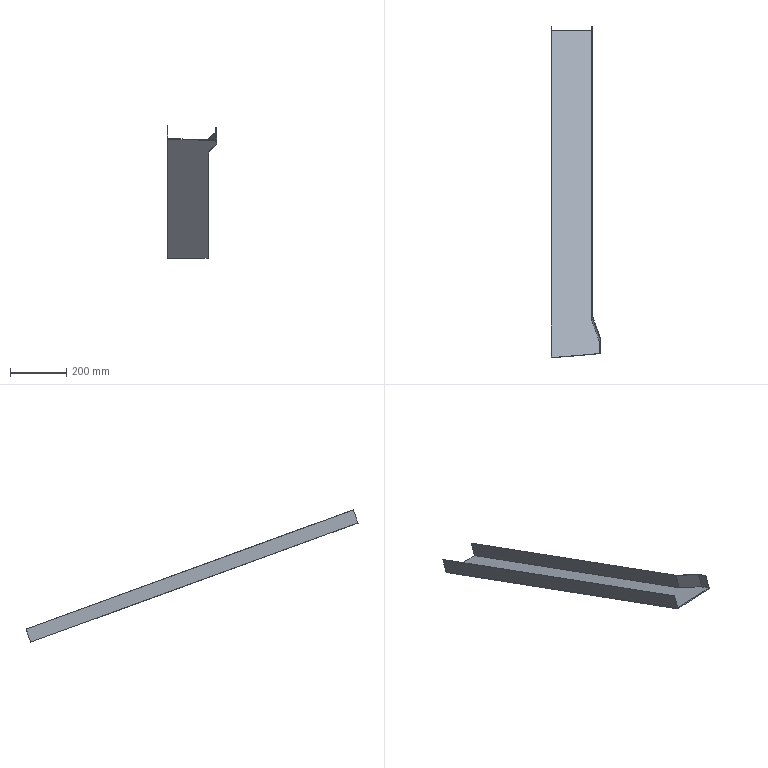Part | NX | features solid 2 | 1 solid | 20 faces | box 175.737 x 1183 x 471.211 mm | volume 600196 mm3 | plane 13 | spline 7
STEP:
#1=CARTESIAN_POINT('',(-1118.,-193.74,-135.956));
#2=VERTEX_POINT('',#1);
#3=CARTESIAN_POINT('',(-1118.,971.638,-560.119));
#4=VERTEX_POINT('',#3);
#5=CARTESIAN_POINT('',(-1118.,-136.156,-156.914));
#6=DIRECTION('',(0.,0.9397,-0.342));
#7=VECTOR('',#6,1000.);
#8=LINE('',#5,#7);
#9=EDGE_CURVE('',#2,#4,#8,.T.);
#10=ORIENTED_EDGE('',*,*,#9,.F.);
#11=CARTESIAN_POINT('',(-945.824,-178.677,-141.438));
#12=VERTEX_POINT('',#11);
#13=CARTESIAN_POINT('',(-1218.424,-202.526,-132.758));
#14=DIRECTION('',(0.9957,0.08711,-0.03171));
#15=VECTOR('',#14,1000.);
#16=LINE('',#13,#15);
#17=EDGE_CURVE('',#2,#12,#16,.T.);
#18=ORIENTED_EDGE('',*,*,#17,.T.);
#19=CARTESIAN_POINT('',(-947.819,-178.548,-141.485));
#20=VERTEX_POINT('',#19);
#21=CARTESIAN_POINT('',(-1226.783,-160.524,-148.045));
#22=DIRECTION('',(0.9976,-0.06446,0.02346));
#23=VECTOR('',#22,1000.);
#24=LINE('',#21,#23);
#25=EDGE_CURVE('',#20,#12,#24,.T.);
#26=ORIENTED_EDGE('',*,*,#25,.F.);
#27=CARTESIAN_POINT('',(-946.331,-142.065,-154.764));
#28=VERTEX_POINT('',#27);
#29=CARTESIAN_POINT('',(-947.819,-178.548,-141.485));
#30=CARTESIAN_POINT('',(-947.597,-175.511,-142.591));
#31=CARTESIAN_POINT('',(-946.951,-169.452,-144.796));
#32=CARTESIAN_POINT('',(-946.188,-157.291,-149.222));
#33=CARTESIAN_POINT('',(-946.239,-148.154,-152.548));
#34=CARTESIAN_POINT('',(-946.331,-142.065,-154.764));
#35=B_SPLINE_CURVE_WITH_KNOTS('',3,(#29,#30,#31,#32,#33,#34),.UNSPECIFIED.,.F.,.F.,(4,1,1,4),(0.,0.009718,0.01944,0.03887),.UNSPECIFIED.);
#36=EDGE_CURVE('',#20,#28,#35,.T.);
#37=ORIENTED_EDGE('',*,*,#36,.T.);
#38=CARTESIAN_POINT('',(-977.,-57.802,-185.433));
#39=VERTEX_POINT('',#38);
#40=CARTESIAN_POINT('',(-977.44,-56.592,-185.873));
#41=DIRECTION('',(-0.3236,0.8891,-0.3236));
#42=VECTOR('',#41,1000.);
#43=LINE('',#40,#42);
#44=EDGE_CURVE('',#28,#39,#43,.T.);
#45=ORIENTED_EDGE('',*,*,#44,.T.);
#46=CARTESIAN_POINT('',(-977.,971.638,-560.119));
#47=VERTEX_POINT('',#46);
#48=CARTESIAN_POINT('',(-977.,-136.156,-156.914));
#49=DIRECTION('',(0.,0.9397,-0.342));
#50=VECTOR('',#49,1000.);
#51=LINE('',#48,#50);
#52=EDGE_CURVE('',#39,#47,#51,.T.);
#53=ORIENTED_EDGE('',*,*,#52,.T.);
#54=CARTESIAN_POINT('',(-1100.,971.638,-560.119));
#55=DIRECTION('',(1.,0.,0.));
#56=VECTOR('',#55,1000.);
#57=LINE('',#54,#56);
#58=EDGE_CURVE('',#4,#47,#57,.T.);
#59=ORIENTED_EDGE('',*,*,#58,.F.);
#60=EDGE_LOOP('',(#10,#18,#26,#37,#45,#53,#59));
#61=FACE_BOUND('',#60,.T.);
#62=CARTESIAN_POINT('',(-1225.,-136.156,-156.914));
#63=DIRECTION('',(0.,-0.342,-0.9397));
#64=DIRECTION('',(0.,0.9397,-0.342));
#65=AXIS2_PLACEMENT_3D('',#62,#63,#64);
#66=PLANE('',#65);
#67=ADVANCED_FACE('',(#61),#66,.F.);
#68=CARTESIAN_POINT('',(-1118.,-194.424,-137.835));
#69=VERTEX_POINT('',#68);
#70=CARTESIAN_POINT('',(-1118.,-194.424,-137.835));
#71=DIRECTION('',(0.,0.342,0.9397));
#72=VECTOR('',#71,1000.);
#73=LINE('',#70,#72);
#74=EDGE_CURVE('',#69,#2,#73,.T.);
#75=ORIENTED_EDGE('',*,*,#74,.F.);
#76=CARTESIAN_POINT('',(-945.824,-179.361,-143.318));
#77=VERTEX_POINT('',#76);
#78=CARTESIAN_POINT('',(-1218.424,-203.21,-134.637));
#79=DIRECTION('',(0.9957,0.08711,-0.03171));
#80=VECTOR('',#79,1000.);
#81=LINE('',#78,#80);
#82=EDGE_CURVE('',#69,#77,#81,.T.);
#83=ORIENTED_EDGE('',*,*,#82,.T.);
#84=CARTESIAN_POINT('',(-945.824,-179.019,-142.378));
#85=DIRECTION('',(0.,0.342,0.9397));
#86=VECTOR('',#85,1000.);
#87=LINE('',#84,#86);
#88=EDGE_CURVE('',#77,#12,#87,.T.);
#89=ORIENTED_EDGE('',*,*,#88,.T.);
#90=ORIENTED_EDGE('',*,*,#17,.F.);
#91=EDGE_LOOP('',(#75,#83,#89,#90));
#92=FACE_BOUND('',#91,.T.);
#93=CARTESIAN_POINT('',(-1218.424,-203.21,-134.637));
#94=DIRECTION('',(-0.0927,0.9356,-0.3405));
#95=DIRECTION('',(0.,0.342,0.9397));
#96=AXIS2_PLACEMENT_3D('',#93,#94,#95);
#97=PLANE('',#96);
#98=ADVANCED_FACE('',(#92),#97,.F.);
#99=CARTESIAN_POINT('',(-944.358,-157.689,-149.077));
#100=VERTEX_POINT('',#99);
#101=CARTESIAN_POINT('',(-944.358,-158.364,-150.96));
#102=VERTEX_POINT('',#101);
#103=CARTESIAN_POINT('',(-944.358,-141.272,-103.972));
#104=DIRECTION('',(0.,-0.342,-0.9397));
#105=VECTOR('',#104,1000.);
#106=LINE('',#103,#105);
#107=EDGE_CURVE('',#100,#102,#106,.T.);
#108=ORIENTED_EDGE('',*,*,#107,.F.);
#109=CARTESIAN_POINT('',(-945.,-169.316,-144.845));
#110=VERTEX_POINT('',#109);
#111=CARTESIAN_POINT('',(-945.,-169.316,-144.845));
#112=CARTESIAN_POINT('',(-944.911,-168.24,-145.237));
#113=CARTESIAN_POINT('',(-944.751,-166.152,-145.997));
#114=CARTESIAN_POINT('',(-944.614,-164.006,-146.778));
#115=CARTESIAN_POINT('',(-944.536,-162.589,-147.294));
#116=CARTESIAN_POINT('',(-944.496,-161.793,-147.584));
#117=CARTESIAN_POINT('',(-944.431,-160.279,-148.135));
#118=CARTESIAN_POINT('',(-944.385,-158.779,-148.68));
#119=CARTESIAN_POINT('',(-944.358,-157.689,-149.077));
#120=B_SPLINE_CURVE_WITH_KNOTS('',3,(#111,#112,#113,#114,#115,#116,#117,#118,#119),.UNSPECIFIED.,.F.,.F.,(4,1,1,1,1,1,4),(0.,0.1082,0.2163,0.2434,0.2704,0.3245,0.4327),.UNSPECIFIED.);
#121=EDGE_CURVE('',#110,#100,#120,.T.);
#122=ORIENTED_EDGE('',*,*,#121,.F.);
#123=CARTESIAN_POINT('',(-945.,-170.,-146.725));
#124=VERTEX_POINT('',#123);
#125=CARTESIAN_POINT('',(-945.,-170.,-146.725));
#126=CARTESIAN_POINT('',(-945.,-169.772,-146.098));
#127=CARTESIAN_POINT('',(-945.,-169.544,-145.472));
#128=CARTESIAN_POINT('',(-945.,-169.316,-144.845));
#129=B_SPLINE_CURVE_WITH_KNOTS('',3,(#125,#126,#127,#128),.UNSPECIFIED.,.F.,.F.,(4,4),(0.,1.),.UNSPECIFIED.);
#130=EDGE_CURVE('',#124,#110,#129,.T.);
#131=ORIENTED_EDGE('',*,*,#130,.F.);
#132=CARTESIAN_POINT('',(-945.,-170.,-146.725));
#133=CARTESIAN_POINT('',(-944.911,-168.923,-147.117));
#134=CARTESIAN_POINT('',(-944.751,-166.834,-147.877));
#135=CARTESIAN_POINT('',(-944.613,-164.687,-148.659));
#136=CARTESIAN_POINT('',(-944.536,-163.269,-149.175));
#137=CARTESIAN_POINT('',(-944.496,-162.473,-149.464));
#138=CARTESIAN_POINT('',(-944.431,-160.956,-150.016));
#139=CARTESIAN_POINT('',(-944.385,-159.455,-150.563));
#140=CARTESIAN_POINT('',(-944.358,-158.364,-150.96));
#141=B_SPLINE_CURVE_WITH_KNOTS('',3,(#132,#133,#134,#135,#136,#137,#138,#139,#140),.UNSPECIFIED.,.F.,.F.,(4,1,1,1,1,1,4),(0.,0.1082,0.2165,0.2435,0.2706,0.3247,0.433),.UNSPECIFIED.);
#142=EDGE_CURVE('',#102,#124,#141,.F.);
#143=ORIENTED_EDGE('',*,*,#142,.F.);
#144=EDGE_LOOP('',(#108,#122,#131,#143));
#145=FACE_BOUND('',#144,.T.);
#146=CARTESIAN_POINT('',(-945.,-170.,-146.725));
#147=CARTESIAN_POINT('',(-945.,-169.316,-144.845));
#148=CARTESIAN_POINT('',(-944.91,-168.917,-147.119));
#149=CARTESIAN_POINT('',(-944.91,-168.233,-145.24));
#150=CARTESIAN_POINT('',(-944.749,-166.815,-147.884));
#151=CARTESIAN_POINT('',(-944.749,-166.131,-146.005));
#152=CARTESIAN_POINT('',(-944.612,-164.658,-148.669));
#153=CARTESIAN_POINT('',(-944.612,-163.974,-146.79));
#154=CARTESIAN_POINT('',(-944.534,-163.231,-149.188));
#155=CARTESIAN_POINT('',(-944.534,-162.547,-147.309));
#156=CARTESIAN_POINT('',(-944.494,-162.438,-149.477));
#157=CARTESIAN_POINT('',(-944.494,-161.754,-147.598));
#158=CARTESIAN_POINT('',(-944.429,-160.9,-150.037));
#159=CARTESIAN_POINT('',(-944.429,-160.216,-148.157));
#160=CARTESIAN_POINT('',(-944.383,-159.388,-150.587));
#161=CARTESIAN_POINT('',(-944.383,-158.704,-148.708));
#162=CARTESIAN_POINT('',(-944.356,-158.286,-150.988));
#163=CARTESIAN_POINT('',(-944.356,-157.602,-149.109));
#164=B_SPLINE_SURFACE_WITH_KNOTS('',3,1,((#146,#147),(#148,#149),(#150,#151),(#152,#153),(#154,#155),(#156,#157),(#158,#159),(#160,#161),(#162,#163)),.SURF_OF_LINEAR_EXTRUSION.,.F.,.F.,.F.,(4,1,1,1,1,1,4),(2,2),(0.,0.1089,0.2178,0.245,0.2722,0.3267,0.4356),(0.,1.),.UNSPECIFIED.);
#165=ADVANCED_FACE('',(#145),#164,.T.);
#166=CARTESIAN_POINT('',(-975.,-58.173,-187.426));
#167=VERTEX_POINT('',#166);
#168=CARTESIAN_POINT('',(-975.,-41.072,-140.442));
#169=VERTEX_POINT('',#168);
#170=CARTESIAN_POINT('',(-975.,-58.173,-187.426));
#171=DIRECTION('',(0.,0.342,0.9397));
#172=VECTOR('',#171,1000.);
#173=LINE('',#170,#172);
#174=EDGE_CURVE('',#167,#169,#173,.T.);
#175=ORIENTED_EDGE('',*,*,#174,.T.);
#176=CARTESIAN_POINT('',(-944.335,-125.322,-109.777));
#177=VERTEX_POINT('',#176);
#178=CARTESIAN_POINT('',(-944.335,-125.322,-109.777));
#179=CARTESIAN_POINT('',(-954.557,-97.239,-119.999));
#180=CARTESIAN_POINT('',(-964.778,-69.155,-130.22));
#181=CARTESIAN_POINT('',(-975.,-41.072,-140.442));
#182=B_SPLINE_CURVE_WITH_KNOTS('',3,(#178,#179,#180,#181),.UNSPECIFIED.,.F.,.F.,(4,4),(0.03202,0.1091),.PIECEWISE_BEZIER_KNOTS.);
#183=EDGE_CURVE('',#177,#169,#182,.T.);
#184=ORIENTED_EDGE('',*,*,#183,.F.);
#185=CARTESIAN_POINT('',(-944.335,-141.739,-154.883));
#186=VERTEX_POINT('',#185);
#187=CARTESIAN_POINT('',(-944.335,-125.322,-109.777));
#188=DIRECTION('',(0.,-0.342,-0.9397));
#189=VECTOR('',#188,1000.);
#190=LINE('',#187,#189);
#191=EDGE_CURVE('',#177,#186,#190,.T.);
#192=ORIENTED_EDGE('',*,*,#191,.T.);
#193=CARTESIAN_POINT('',(-944.335,-142.423,-156.762));
#194=VERTEX_POINT('',#193);
#195=CARTESIAN_POINT('',(-944.335,-142.423,-156.762));
#196=CARTESIAN_POINT('',(-944.335,-142.195,-156.135));
#197=CARTESIAN_POINT('',(-944.335,-141.967,-155.509));
#198=CARTESIAN_POINT('',(-944.335,-141.739,-154.883));
#199=B_SPLINE_CURVE_WITH_KNOTS('',3,(#195,#196,#197,#198),.UNSPECIFIED.,.F.,.F.,(4,4),(0.,1.),.UNSPECIFIED.);
#200=EDGE_CURVE('',#186,#194,#199,.F.);
#201=ORIENTED_EDGE('',*,*,#200,.T.);
#202=CARTESIAN_POINT('',(-975.548,-56.668,-187.974));
#203=DIRECTION('',(-0.3236,0.8891,-0.3236));
#204=VECTOR('',#203,1000.);
#205=LINE('',#202,#204);
#206=EDGE_CURVE('',#194,#167,#205,.T.);
#207=ORIENTED_EDGE('',*,*,#206,.T.);
#208=EDGE_LOOP('',(#175,#184,#192,#201,#207));
#209=FACE_BOUND('',#208,.T.);
#210=CARTESIAN_POINT('',(-975.548,-56.668,-187.974));
#211=DIRECTION('',(0.9462,0.3041,-0.1107));
#212=DIRECTION('',(-0.306,0.952,0.));
#213=AXIS2_PLACEMENT_3D('',#210,#211,#212);
#214=PLANE('',#213);
#215=ADVANCED_FACE('',(#209),#214,.T.);
#216=CARTESIAN_POINT('',(-975.,970.954,-561.998));
#217=VERTEX_POINT('',#216);
#218=CARTESIAN_POINT('',(-975.,988.055,-515.013));
#219=VERTEX_POINT('',#218);
#220=CARTESIAN_POINT('',(-975.,970.954,-561.998));
#221=DIRECTION('',(0.,0.342,0.9397));
#222=VECTOR('',#221,1000.);
#223=LINE('',#220,#222);
#224=EDGE_CURVE('',#217,#219,#223,.T.);
#225=ORIENTED_EDGE('',*,*,#224,.T.);
#226=CARTESIAN_POINT('',(-975.,-41.072,-140.442));
#227=CARTESIAN_POINT('',(-975.,301.97,-265.299));
#228=CARTESIAN_POINT('',(-975.,645.013,-390.156));
#229=CARTESIAN_POINT('',(-975.,988.055,-515.013));
#230=B_SPLINE_CURVE_WITH_KNOTS('',3,(#226,#227,#228,#229),.UNSPECIFIED.,.F.,.F.,(4,4),(0.1091,1.),.PIECEWISE_BEZIER_KNOTS.);
#231=EDGE_CURVE('',#169,#219,#230,.T.);
#232=ORIENTED_EDGE('',*,*,#231,.F.);
#233=ORIENTED_EDGE('',*,*,#174,.F.);
#234=CARTESIAN_POINT('',(-975.,-136.84,-158.794));
#235=DIRECTION('',(0.,0.9397,-0.342));
#236=VECTOR('',#235,1000.);
#237=LINE('',#234,#236);
#238=EDGE_CURVE('',#167,#217,#237,.T.);
#239=ORIENTED_EDGE('',*,*,#238,.T.);
#240=EDGE_LOOP('',(#225,#232,#233,#239));
#241=FACE_BOUND('',#240,.T.);
#242=CARTESIAN_POINT('',(-975.,-136.84,-158.794));
#243=DIRECTION('',(1.,0.,0.));
#244=DIRECTION('',(0.,0.,-1.));
#245=AXIS2_PLACEMENT_3D('',#242,#243,#244);
#246=PLANE('',#245);
#247=ADVANCED_FACE('',(#241),#246,.T.);
#248=CARTESIAN_POINT('',(-1120.,970.954,-561.998));
#249=VERTEX_POINT('',#248);
#250=CARTESIAN_POINT('',(-1120.,988.055,-515.013));
#251=VERTEX_POINT('',#250);
#252=CARTESIAN_POINT('',(-1120.,970.954,-561.998));
#253=DIRECTION('',(0.,0.342,0.9397));
#254=VECTOR('',#253,1000.);
#255=LINE('',#252,#254);
#256=EDGE_CURVE('',#249,#251,#255,.T.);
#257=ORIENTED_EDGE('',*,*,#256,.T.);
#258=CARTESIAN_POINT('',(-1118.,988.055,-515.013));
#259=VERTEX_POINT('',#258);
#260=CARTESIAN_POINT('',(-1120.,988.055,-515.013));
#261=DIRECTION('',(1.,0.,0.));
#262=VECTOR('',#261,1000.);
#263=LINE('',#260,#262);
#264=EDGE_CURVE('',#251,#259,#263,.T.);
#265=ORIENTED_EDGE('',*,*,#264,.T.);
#266=CARTESIAN_POINT('',(-1118.,988.055,-515.013));
#267=DIRECTION('',(0.,-0.342,-0.9397));
#268=VECTOR('',#267,1000.);
#269=LINE('',#266,#268);
#270=EDGE_CURVE('',#259,#4,#269,.T.);
#271=ORIENTED_EDGE('',*,*,#270,.T.);
#272=ORIENTED_EDGE('',*,*,#58,.T.);
#273=CARTESIAN_POINT('',(-977.,988.055,-515.013));
#274=VERTEX_POINT('',#273);
#275=CARTESIAN_POINT('',(-977.,988.055,-515.013));
#276=DIRECTION('',(0.,-0.342,-0.9397));
#277=VECTOR('',#276,1000.);
#278=LINE('',#275,#277);
#279=EDGE_CURVE('',#274,#47,#278,.T.);
#280=ORIENTED_EDGE('',*,*,#279,.F.);
#281=CARTESIAN_POINT('',(-975.,988.055,-515.013));
#282=DIRECTION('',(1.,0.,0.));
#283=VECTOR('',#282,1000.);
#284=LINE('',#281,#283);
#285=EDGE_CURVE('',#219,#274,#284,.F.);
#286=ORIENTED_EDGE('',*,*,#285,.F.);
#287=ORIENTED_EDGE('',*,*,#224,.F.);
#288=CARTESIAN_POINT('',(-1100.,970.954,-561.998));
#289=DIRECTION('',(1.,0.,0.));
#290=VECTOR('',#289,1000.);
#291=LINE('',#288,#290);
#292=EDGE_CURVE('',#249,#217,#291,.T.);
#293=ORIENTED_EDGE('',*,*,#292,.F.);
#294=EDGE_LOOP('',(#257,#265,#271,#272,#280,#286,#287,#293));
#295=FACE_BOUND('',#294,.T.);
#296=CARTESIAN_POINT('',(-1100.,970.954,-561.998));
#297=DIRECTION('',(0.,-0.9397,0.342));
#298=DIRECTION('',(0.,-0.342,-0.9397));
#299=AXIS2_PLACEMENT_3D('',#296,#297,#298);
#300=PLANE('',#299);
#301=ADVANCED_FACE('',(#295),#300,.F.);
#302=CARTESIAN_POINT('',(-1120.,-194.599,-137.771));
#303=VERTEX_POINT('',#302);
#304=CARTESIAN_POINT('',(-1120.,-177.498,-90.787));
#305=VERTEX_POINT('',#304);
#306=CARTESIAN_POINT('',(-1120.,-194.599,-137.771));
#307=DIRECTION('',(0.,0.342,0.9397));
#308=VECTOR('',#307,1000.);
#309=LINE('',#306,#308);
#310=EDGE_CURVE('',#303,#305,#309,.T.);
#311=ORIENTED_EDGE('',*,*,#310,.T.);
#312=CARTESIAN_POINT('',(-1120.,-177.498,-90.787));
#313=DIRECTION('',(0.,0.9397,-0.342));
#314=VECTOR('',#313,1000.);
#315=LINE('',#312,#314);
#316=EDGE_CURVE('',#305,#251,#315,.T.);
#317=ORIENTED_EDGE('',*,*,#316,.T.);
#318=ORIENTED_EDGE('',*,*,#256,.F.);
#319=CARTESIAN_POINT('',(-1120.,450.045,-372.403));
#320=DIRECTION('',(0.,0.9397,-0.342));
#321=VECTOR('',#320,1000.);
#322=LINE('',#319,#321);
#323=EDGE_CURVE('',#303,#249,#322,.T.);
#324=ORIENTED_EDGE('',*,*,#323,.F.);
#325=EDGE_LOOP('',(#311,#317,#318,#324));
#326=FACE_BOUND('',#325,.T.);
#327=CARTESIAN_POINT('',(-1120.,450.045,-372.403));
#328=DIRECTION('',(1.,0.,0.));
#329=DIRECTION('',(0.,0.,-1.));
#330=AXIS2_PLACEMENT_3D('',#327,#328,#329);
#331=PLANE('',#330);
#332=ADVANCED_FACE('',(#326),#331,.F.);
#333=CARTESIAN_POINT('',(-945.824,-178.677,-141.438));
#334=CARTESIAN_POINT('',(-945.807,-178.456,-141.519));
#335=CARTESIAN_POINT('',(-945.796,-178.3,-141.575));
#336=CARTESIAN_POINT('',(-945.751,-177.74,-141.779));
#337=CARTESIAN_POINT('',(-945.68,-176.921,-142.077));
#338=CARTESIAN_POINT('',(-945.584,-175.837,-142.472));
#339=CARTESIAN_POINT('',(-945.494,-174.858,-142.828));
#340=CARTESIAN_POINT('',(-945.387,-173.696,-143.251));
#341=CARTESIAN_POINT('',(-945.295,-172.711,-143.61));
#342=CARTESIAN_POINT('',(-945.147,-171.057,-144.212));
#343=CARTESIAN_POINT('',(-945.055,-169.984,-144.602));
#344=CARTESIAN_POINT('',(-945.,-169.316,-144.845));
#345=B_SPLINE_CURVE_WITH_KNOTS('',3,(#333,#334,#335,#336,#337,#338,#339,#340,#341,#342,#343,#344),.UNSPECIFIED.,.F.,.F.,(4,1,1,1,1,1,1,1,1,4),(0.493,0.5247,0.5563,0.6197,0.6831,0.7148,0.7465,0.8099,0.8732,1.),.UNSPECIFIED.);
#346=EDGE_CURVE('',#12,#110,#345,.T.);
#347=ORIENTED_EDGE('',*,*,#346,.F.);
#348=ORIENTED_EDGE('',*,*,#88,.F.);
#349=CARTESIAN_POINT('',(-945.824,-179.361,-143.318));
#350=CARTESIAN_POINT('',(-945.807,-179.14,-143.398));
#351=CARTESIAN_POINT('',(-945.796,-178.984,-143.455));
#352=CARTESIAN_POINT('',(-945.751,-178.424,-143.659));
#353=CARTESIAN_POINT('',(-945.68,-177.605,-143.957));
#354=CARTESIAN_POINT('',(-945.584,-176.521,-144.351));
#355=CARTESIAN_POINT('',(-945.494,-175.542,-144.707));
#356=CARTESIAN_POINT('',(-945.387,-174.38,-145.131));
#357=CARTESIAN_POINT('',(-945.295,-173.395,-145.489));
#358=CARTESIAN_POINT('',(-945.147,-171.741,-146.091));
#359=CARTESIAN_POINT('',(-945.055,-170.668,-146.481));
#360=CARTESIAN_POINT('',(-945.,-170.,-146.725));
#361=B_SPLINE_CURVE_WITH_KNOTS('',3,(#349,#350,#351,#352,#353,#354,#355,#356,#357,#358,#359,#360),.UNSPECIFIED.,.F.,.F.,(4,1,1,1,1,1,1,1,1,4),(0.493,0.5247,0.5563,0.6197,0.6831,0.7148,0.7465,0.8099,0.8732,1.),.UNSPECIFIED.);
#362=EDGE_CURVE('',#77,#124,#361,.T.);
#363=ORIENTED_EDGE('',*,*,#362,.T.);
#364=ORIENTED_EDGE('',*,*,#130,.T.);
#365=EDGE_LOOP('',(#347,#348,#363,#364));
#366=FACE_BOUND('',#365,.T.);
#367=CARTESIAN_POINT('',(-945.824,-179.361,-143.318));
#368=CARTESIAN_POINT('',(-945.824,-178.677,-141.438));
#369=CARTESIAN_POINT('',(-945.807,-179.14,-143.398));
#370=CARTESIAN_POINT('',(-945.807,-178.456,-141.519));
#371=CARTESIAN_POINT('',(-945.796,-178.984,-143.455));
#372=CARTESIAN_POINT('',(-945.796,-178.3,-141.575));
#373=CARTESIAN_POINT('',(-945.751,-178.424,-143.659));
#374=CARTESIAN_POINT('',(-945.751,-177.74,-141.779));
#375=CARTESIAN_POINT('',(-945.68,-177.605,-143.957));
#376=CARTESIAN_POINT('',(-945.68,-176.921,-142.077));
#377=CARTESIAN_POINT('',(-945.584,-176.521,-144.351));
#378=CARTESIAN_POINT('',(-945.584,-175.837,-142.472));
#379=CARTESIAN_POINT('',(-945.494,-175.542,-144.707));
#380=CARTESIAN_POINT('',(-945.494,-174.858,-142.828));
#381=CARTESIAN_POINT('',(-945.387,-174.38,-145.131));
#382=CARTESIAN_POINT('',(-945.387,-173.696,-143.251));
#383=CARTESIAN_POINT('',(-945.295,-173.395,-145.489));
#384=CARTESIAN_POINT('',(-945.295,-172.711,-143.61));
#385=CARTESIAN_POINT('',(-945.147,-171.741,-146.091));
#386=CARTESIAN_POINT('',(-945.147,-171.057,-144.212));
#387=CARTESIAN_POINT('',(-945.055,-170.668,-146.481));
#388=CARTESIAN_POINT('',(-945.055,-169.984,-144.602));
#389=CARTESIAN_POINT('',(-945.,-170.,-146.725));
#390=CARTESIAN_POINT('',(-945.,-169.316,-144.845));
#391=B_SPLINE_SURFACE_WITH_KNOTS('',3,1,((#367,#368),(#369,#370),(#371,#372),(#373,#374),(#375,#376),(#377,#378),(#379,#380),(#381,#382),(#383,#384),(#385,#386),(#387,#388),(#389,#390)),.SURF_OF_LINEAR_EXTRUSION.,.F.,.F.,.F.,(4,1,1,1,1,1,1,1,1,4),(2,2),(0.493,0.5247,0.5563,0.6197,0.6831,0.7148,0.7465,0.8099,0.8732,1.),(0.,1.),.UNSPECIFIED.);
#392=ADVANCED_FACE('',(#366),#391,.T.);
#393=ORIENTED_EDGE('',*,*,#292,.T.);
#394=ORIENTED_EDGE('',*,*,#238,.F.);
#395=ORIENTED_EDGE('',*,*,#206,.F.);
#396=CARTESIAN_POINT('',(-944.358,-158.364,-150.96));
#397=CARTESIAN_POINT('',(-944.349,-158.007,-151.09));
#398=CARTESIAN_POINT('',(-944.333,-157.298,-151.348));
#399=CARTESIAN_POINT('',(-944.313,-156.241,-151.733));
#400=CARTESIAN_POINT('',(-944.305,-155.742,-151.914));
#401=CARTESIAN_POINT('',(-944.296,-155.173,-152.121));
#402=CARTESIAN_POINT('',(-944.284,-154.187,-152.48));
#403=CARTESIAN_POINT('',(-944.271,-152.704,-153.02));
#404=CARTESIAN_POINT('',(-944.26,-148.971,-154.379));
#405=CARTESIAN_POINT('',(-944.288,-145.47,-155.653));
#406=CARTESIAN_POINT('',(-944.335,-142.423,-156.762));
#407=B_SPLINE_CURVE_WITH_KNOTS('',3,(#396,#397,#398,#399,#400,#401,#402,#403,#404,#405,#406),.UNSPECIFIED.,.F.,.F.,(4,1,1,1,1,1,1,1,4),(0.433,0.4684,0.5038,0.5216,0.5393,0.5747,0.6456,0.7165,1.),.UNSPECIFIED.);
#408=EDGE_CURVE('',#194,#102,#407,.F.);
#409=ORIENTED_EDGE('',*,*,#408,.T.);
#410=ORIENTED_EDGE('',*,*,#142,.T.);
#411=ORIENTED_EDGE('',*,*,#362,.F.);
#412=ORIENTED_EDGE('',*,*,#82,.F.);
#413=CARTESIAN_POINT('',(-1118.,-194.599,-137.771));
#414=VERTEX_POINT('',#413);
#415=CARTESIAN_POINT('',(-1118.,-194.599,-137.771));
#416=DIRECTION('',(0.,0.9397,-0.342));
#417=VECTOR('',#416,1000.);
#418=LINE('',#415,#417);
#419=EDGE_CURVE('',#414,#69,#418,.T.);
#420=ORIENTED_EDGE('',*,*,#419,.F.);
#421=CARTESIAN_POINT('',(-1120.,-194.599,-137.771));
#422=DIRECTION('',(1.,0.,0.));
#423=VECTOR('',#422,1000.);
#424=LINE('',#421,#423);
#425=EDGE_CURVE('',#303,#414,#424,.T.);
#426=ORIENTED_EDGE('',*,*,#425,.F.);
#427=ORIENTED_EDGE('',*,*,#323,.T.);
#428=EDGE_LOOP('',(#393,#394,#395,#409,#410,#411,#412,#420,#426,#427));
#429=FACE_BOUND('',#428,.T.);
#430=CARTESIAN_POINT('',(-1225.,-136.84,-158.794));
#431=DIRECTION('',(0.,-0.342,-0.9397));
#432=DIRECTION('',(0.,0.9397,-0.342));
#433=AXIS2_PLACEMENT_3D('',#430,#431,#432);
#434=PLANE('',#433);
#435=ADVANCED_FACE('',(#429),#434,.T.);
#436=CARTESIAN_POINT('',(-947.819,-162.131,-96.38));
#437=VERTEX_POINT('',#436);
#438=CARTESIAN_POINT('',(-947.819,-162.131,-96.38));
#439=DIRECTION('',(0.,-0.342,-0.9397));
#440=VECTOR('',#439,1000.);
#441=LINE('',#438,#440);
#442=EDGE_CURVE('',#437,#20,#441,.T.);
#443=ORIENTED_EDGE('',*,*,#442,.T.);
#444=ORIENTED_EDGE('',*,*,#25,.T.);
#445=CARTESIAN_POINT('',(-945.824,-162.26,-96.333));
#446=VERTEX_POINT('',#445);
#447=CARTESIAN_POINT('',(-945.824,-162.26,-96.333));
#448=DIRECTION('',(0.,-0.342,-0.9397));
#449=VECTOR('',#448,1000.);
#450=LINE('',#447,#449);
#451=EDGE_CURVE('',#446,#12,#450,.T.);
#452=ORIENTED_EDGE('',*,*,#451,.F.);
#453=CARTESIAN_POINT('',(-947.819,-162.131,-96.38));
#454=CARTESIAN_POINT('',(-947.154,-162.174,-96.364));
#455=CARTESIAN_POINT('',(-946.489,-162.217,-96.349));
#456=CARTESIAN_POINT('',(-945.824,-162.26,-96.333));
#457=B_SPLINE_CURVE_WITH_KNOTS('',3,(#453,#454,#455,#456),.UNSPECIFIED.,.F.,.F.,(4,4),(0.,1.),.UNSPECIFIED.);
#458=EDGE_CURVE('',#446,#437,#457,.F.);
#459=ORIENTED_EDGE('',*,*,#458,.T.);
#460=EDGE_LOOP('',(#443,#444,#452,#459));
#461=FACE_BOUND('',#460,.T.);
#462=CARTESIAN_POINT('',(-945.824,-162.26,-96.333));
#463=DIRECTION('',(0.06859,0.9375,-0.3412));
#464=DIRECTION('',(0.,-0.342,-0.9397));
#465=AXIS2_PLACEMENT_3D('',#462,#463,#464);
#466=PLANE('',#465);
#467=ADVANCED_FACE('',(#461),#466,.F.);
#468=ORIENTED_EDGE('',*,*,#36,.F.);
#469=ORIENTED_EDGE('',*,*,#442,.F.);
#470=CARTESIAN_POINT('',(-946.331,-125.648,-109.659));
#471=VERTEX_POINT('',#470);
#472=CARTESIAN_POINT('',(-947.819,-162.131,-96.38));
#473=CARTESIAN_POINT('',(-947.808,-161.978,-96.436));
#474=CARTESIAN_POINT('',(-947.801,-161.885,-96.469));
#475=CARTESIAN_POINT('',(-947.78,-161.61,-96.569));
#476=CARTESIAN_POINT('',(-947.749,-161.238,-96.705));
#477=CARTESIAN_POINT('',(-947.704,-160.699,-96.901));
#478=CARTESIAN_POINT('',(-947.631,-159.872,-97.202));
#479=CARTESIAN_POINT('',(-947.542,-158.879,-97.564));
#480=CARTESIAN_POINT('',(-947.448,-157.858,-97.935));
#481=CARTESIAN_POINT('',(-947.39,-157.239,-98.16));
#482=CARTESIAN_POINT('',(-947.327,-156.559,-98.408));
#483=CARTESIAN_POINT('',(-947.23,-155.496,-98.795));
#484=CARTESIAN_POINT('',(-947.081,-153.801,-99.412));
#485=CARTESIAN_POINT('',(-946.927,-151.969,-100.079));
#486=CARTESIAN_POINT('',(-946.765,-149.787,-100.873));
#487=CARTESIAN_POINT('',(-946.579,-146.871,-101.934));
#488=CARTESIAN_POINT('',(-946.336,-141.769,-103.791));
#489=CARTESIAN_POINT('',(-946.225,-134.457,-106.453));
#490=CARTESIAN_POINT('',(-946.286,-128.587,-108.589));
#491=CARTESIAN_POINT('',(-946.331,-125.648,-109.659));
#492=B_SPLINE_CURVE_WITH_KNOTS('',3,(#472,#473,#474,#475,#476,#477,#478,#479,#480,#481,#482,#483,#484,#485,#486,#487,#488,#489,#490,#491),.UNSPECIFIED.,.F.,.F.,(4,1,1,1,1,1,1,1,1,1,1,1,1,1,1,1,1,4),(0.,0.007812,0.01562,0.03125,0.04688,0.0625,0.09375,0.1094,0.1172,0.125,0.1562,0.1875,0.25,0.3125,0.375,0.5,0.75,1.),.UNSPECIFIED.);
#493=EDGE_CURVE('',#437,#471,#492,.T.);
#494=ORIENTED_EDGE('',*,*,#493,.T.);
#495=CARTESIAN_POINT('',(-946.331,-134.198,-133.151));
#496=DIRECTION('',(0.,-0.342,-0.9397));
#497=VECTOR('',#496,1000.);
#498=LINE('',#495,#497);
#499=EDGE_CURVE('',#471,#28,#498,.T.);
#500=ORIENTED_EDGE('',*,*,#499,.T.);
#501=EDGE_LOOP('',(#468,#469,#494,#500));
#502=FACE_BOUND('',#501,.T.);
#503=CARTESIAN_POINT('',(-947.819,-162.131,-96.38));
#504=CARTESIAN_POINT('',(-947.819,-178.548,-141.485));
#505=CARTESIAN_POINT('',(-947.801,-161.886,-96.469));
#506=CARTESIAN_POINT('',(-947.801,-178.303,-141.574));
#507=CARTESIAN_POINT('',(-947.788,-161.716,-96.531));
#508=CARTESIAN_POINT('',(-947.788,-178.133,-141.636));
#509=CARTESIAN_POINT('',(-947.749,-161.23,-96.708));
#510=CARTESIAN_POINT('',(-947.749,-177.647,-141.813));
#511=CARTESIAN_POINT('',(-947.704,-160.701,-96.9));
#512=CARTESIAN_POINT('',(-947.704,-177.118,-142.006));
#513=CARTESIAN_POINT('',(-947.631,-159.871,-97.202));
#514=CARTESIAN_POINT('',(-947.631,-176.288,-142.308));
#515=CARTESIAN_POINT('',(-947.542,-158.878,-97.564));
#516=CARTESIAN_POINT('',(-947.542,-175.295,-142.669));
#517=CARTESIAN_POINT('',(-947.448,-157.86,-97.934));
#518=CARTESIAN_POINT('',(-947.448,-174.277,-143.04));
#519=CARTESIAN_POINT('',(-947.39,-157.237,-98.161));
#520=CARTESIAN_POINT('',(-947.39,-173.654,-143.266));
#521=CARTESIAN_POINT('',(-947.328,-156.562,-98.407));
#522=CARTESIAN_POINT('',(-947.328,-172.979,-143.512));
#523=CARTESIAN_POINT('',(-947.23,-155.494,-98.795));
#524=CARTESIAN_POINT('',(-947.23,-171.911,-143.901));
#525=CARTESIAN_POINT('',(-947.081,-153.801,-99.412));
#526=CARTESIAN_POINT('',(-947.081,-170.218,-144.517));
#527=CARTESIAN_POINT('',(-946.927,-151.969,-100.079));
#528=CARTESIAN_POINT('',(-946.927,-168.386,-145.184));
#529=CARTESIAN_POINT('',(-946.765,-149.786,-100.873));
#530=CARTESIAN_POINT('',(-946.765,-166.203,-145.978));
#531=CARTESIAN_POINT('',(-946.578,-146.87,-101.934));
#532=CARTESIAN_POINT('',(-946.578,-163.287,-147.04));
#533=CARTESIAN_POINT('',(-946.336,-141.769,-103.791));
#534=CARTESIAN_POINT('',(-946.336,-158.186,-148.896));
#535=CARTESIAN_POINT('',(-946.228,-134.459,-106.452));
#536=CARTESIAN_POINT('',(-946.228,-150.876,-151.557));
#537=CARTESIAN_POINT('',(-946.286,-128.586,-108.589));
#538=CARTESIAN_POINT('',(-946.286,-145.003,-153.695));
#539=CARTESIAN_POINT('',(-946.331,-125.648,-109.659));
#540=CARTESIAN_POINT('',(-946.331,-142.065,-154.764));
#541=B_SPLINE_SURFACE_WITH_KNOTS('',3,1,((#503,#504),(#505,#506),(#507,#508),(#509,#510),(#511,#512),(#513,#514),(#515,#516),(#517,#518),(#519,#520),(#521,#522),(#523,#524),(#525,#526),(#527,#528),(#529,#530),(#531,#532),(#533,#534),(#535,#536),(#537,#538),(#539,#540)),.SURF_OF_LINEAR_EXTRUSION.,.F.,.F.,.F.,(4,1,1,1,1,1,1,1,1,1,1,1,1,1,1,1,4),(2,2),(0.,0.0004961,0.0009922,0.001488,0.001984,0.002977,0.003473,0.003721,0.003969,0.004961,0.005953,0.007938,0.009922,0.01191,0.01588,0.02381,0.03175),(0.,1.),.UNSPECIFIED.);
#542=ADVANCED_FACE('',(#502),#541,.T.);
#543=ORIENTED_EDGE('',*,*,#44,.F.);
#544=ORIENTED_EDGE('',*,*,#499,.F.);
#545=CARTESIAN_POINT('',(-977.,-41.385,-140.328));
#546=VERTEX_POINT('',#545);
#547=CARTESIAN_POINT('',(-941.628,-138.568,-104.956));
#548=CARTESIAN_POINT('',(-943.161,-134.355,-106.489));
#549=CARTESIAN_POINT('',(-944.695,-130.143,-108.023));
#550=CARTESIAN_POINT('',(-946.228,-125.93,-109.556));
#551=CARTESIAN_POINT('',(-956.449,-97.847,-119.777));
#552=CARTESIAN_POINT('',(-966.671,-69.764,-129.999));
#553=CARTESIAN_POINT('',(-976.892,-41.68,-140.22));
#554=CARTESIAN_POINT('',(-978.426,-37.468,-141.754));
#555=CARTESIAN_POINT('',(-979.959,-33.255,-143.287));
#556=CARTESIAN_POINT('',(-981.492,-29.043,-144.82));
#557=B_SPLINE_CURVE_WITH_KNOTS('',3,(#547,#548,#549,#550,#551,#552,#553,#554,#555,#556),.UNSPECIFIED.,.F.,.F.,(4,3,3,4),(0.02046,0.03202,0.1091,0.1207),.PIECEWISE_BEZIER_KNOTS.);
#558=EDGE_CURVE('',#471,#546,#557,.T.);
#559=ORIENTED_EDGE('',*,*,#558,.T.);
#560=CARTESIAN_POINT('',(-977.,-41.385,-140.328));
#561=DIRECTION('',(0.,-0.342,-0.9397));
#562=VECTOR('',#561,1000.);
#563=LINE('',#560,#562);
#564=EDGE_CURVE('',#546,#39,#563,.T.);
#565=ORIENTED_EDGE('',*,*,#564,.T.);
#566=EDGE_LOOP('',(#543,#544,#559,#565));
#567=FACE_BOUND('',#566,.T.);
#568=CARTESIAN_POINT('',(-946.228,-125.93,-109.556));
#569=DIRECTION('',(-0.9462,-0.3041,0.1107));
#570=DIRECTION('',(0.306,-0.952,0.));
#571=AXIS2_PLACEMENT_3D('',#568,#569,#570);
#572=PLANE('',#571);
#573=ADVANCED_FACE('',(#567),#572,.T.);
#574=ORIENTED_EDGE('',*,*,#52,.F.);
#575=ORIENTED_EDGE('',*,*,#564,.F.);
#576=CARTESIAN_POINT('',(-977.,-195.441,-84.256));
#577=CARTESIAN_POINT('',(-977.,-143.985,-102.985));
#578=CARTESIAN_POINT('',(-977.,-92.528,-121.713));
#579=CARTESIAN_POINT('',(-977.,-41.072,-140.442));
#580=CARTESIAN_POINT('',(-977.,301.97,-265.299));
#581=CARTESIAN_POINT('',(-977.,645.013,-390.156));
#582=CARTESIAN_POINT('',(-977.,988.055,-515.013));
#583=CARTESIAN_POINT('',(-977.,1039.511,-533.742));
#584=CARTESIAN_POINT('',(-977.,1090.968,-552.471));
#585=CARTESIAN_POINT('',(-977.,1142.424,-571.199));
#586=B_SPLINE_CURVE_WITH_KNOTS('',3,(#576,#577,#578,#579,#580,#581,#582,#583,#584,#585),.UNSPECIFIED.,.F.,.F.,(4,3,3,4),(-0.02453,0.1091,1.,1.134),.PIECEWISE_BEZIER_KNOTS.);
#587=EDGE_CURVE('',#546,#274,#586,.T.);
#588=ORIENTED_EDGE('',*,*,#587,.T.);
#589=ORIENTED_EDGE('',*,*,#279,.T.);
#590=EDGE_LOOP('',(#574,#575,#588,#589));
#591=FACE_BOUND('',#590,.T.);
#592=CARTESIAN_POINT('',(-977.,-41.072,-140.442));
#593=DIRECTION('',(-1.,0.,0.));
#594=DIRECTION('',(0.,0.,1.));
#595=AXIS2_PLACEMENT_3D('',#592,#593,#594);
#596=PLANE('',#595);
#597=ADVANCED_FACE('',(#591),#596,.T.);
#598=ORIENTED_EDGE('',*,*,#200,.F.);
#599=ORIENTED_EDGE('',*,*,#191,.F.);
#600=CARTESIAN_POINT('',(-945.824,-162.26,-96.333));
#601=CARTESIAN_POINT('',(-945.806,-162.015,-96.422));
#602=CARTESIAN_POINT('',(-945.793,-161.853,-96.481));
#603=CARTESIAN_POINT('',(-945.754,-161.368,-96.658));
#604=CARTESIAN_POINT('',(-945.709,-160.839,-96.85));
#605=CARTESIAN_POINT('',(-945.636,-160.002,-97.155));
#606=CARTESIAN_POINT('',(-945.546,-159.008,-97.517));
#607=CARTESIAN_POINT('',(-945.45,-157.96,-97.898));
#608=CARTESIAN_POINT('',(-945.394,-157.358,-98.117));
#609=CARTESIAN_POINT('',(-945.33,-156.668,-98.368));
#610=CARTESIAN_POINT('',(-945.232,-155.598,-98.758));
#611=CARTESIAN_POINT('',(-945.082,-153.888,-99.38));
#612=CARTESIAN_POINT('',(-944.927,-152.037,-100.054));
#613=CARTESIAN_POINT('',(-944.762,-149.815,-100.863));
#614=CARTESIAN_POINT('',(-944.574,-146.85,-101.942));
#615=CARTESIAN_POINT('',(-944.332,-141.657,-103.832));
#616=CARTESIAN_POINT('',(-944.228,-134.232,-106.534));
#617=CARTESIAN_POINT('',(-944.289,-128.292,-108.696));
#618=CARTESIAN_POINT('',(-944.335,-125.322,-109.777));
#619=B_SPLINE_CURVE_WITH_KNOTS('',3,(#600,#601,#602,#603,#604,#605,#606,#607,#608,#609,#610,#611,#612,#613,#614,#615,#616,#617,#618),.UNSPECIFIED.,.F.,.F.,(4,1,1,1,1,1,1,1,1,1,1,1,1,1,1,1,4),(0.,0.01562,0.03125,0.04688,0.0625,0.09375,0.1094,0.1172,0.125,0.1562,0.1875,0.25,0.3125,0.375,0.5,0.75,1.),.UNSPECIFIED.);
#620=EDGE_CURVE('',#446,#177,#619,.T.);
#621=ORIENTED_EDGE('',*,*,#620,.F.);
#622=ORIENTED_EDGE('',*,*,#451,.T.);
#623=ORIENTED_EDGE('',*,*,#346,.T.);
#624=ORIENTED_EDGE('',*,*,#121,.T.);
#625=ORIENTED_EDGE('',*,*,#107,.T.);
#626=ORIENTED_EDGE('',*,*,#408,.F.);
#627=EDGE_LOOP('',(#598,#599,#621,#622,#623,#624,#625,#626));
#628=FACE_BOUND('',#627,.T.);
#629=CARTESIAN_POINT('',(-945.824,-162.26,-96.333));
#630=CARTESIAN_POINT('',(-945.824,-179.361,-143.318));
#631=CARTESIAN_POINT('',(-945.806,-162.015,-96.422));
#632=CARTESIAN_POINT('',(-945.806,-179.116,-143.407));
#633=CARTESIAN_POINT('',(-945.793,-161.853,-96.481));
#634=CARTESIAN_POINT('',(-945.793,-178.954,-143.466));
#635=CARTESIAN_POINT('',(-945.754,-161.368,-96.658));
#636=CARTESIAN_POINT('',(-945.754,-178.469,-143.642));
#637=CARTESIAN_POINT('',(-945.709,-160.839,-96.85));
#638=CARTESIAN_POINT('',(-945.709,-177.94,-143.835));
#639=CARTESIAN_POINT('',(-945.636,-160.002,-97.155));
#640=CARTESIAN_POINT('',(-945.636,-177.103,-144.139));
#641=CARTESIAN_POINT('',(-945.546,-159.008,-97.517));
#642=CARTESIAN_POINT('',(-945.546,-176.109,-144.501));
#643=CARTESIAN_POINT('',(-945.45,-157.96,-97.898));
#644=CARTESIAN_POINT('',(-945.45,-175.061,-144.883));
#645=CARTESIAN_POINT('',(-945.394,-157.358,-98.117));
#646=CARTESIAN_POINT('',(-945.394,-174.459,-145.102));
#647=CARTESIAN_POINT('',(-945.33,-156.668,-98.368));
#648=CARTESIAN_POINT('',(-945.33,-173.769,-145.353));
#649=CARTESIAN_POINT('',(-945.232,-155.598,-98.758));
#650=CARTESIAN_POINT('',(-945.232,-172.699,-145.742));
#651=CARTESIAN_POINT('',(-945.082,-153.888,-99.38));
#652=CARTESIAN_POINT('',(-945.082,-170.989,-146.365));
#653=CARTESIAN_POINT('',(-944.927,-152.037,-100.054));
#654=CARTESIAN_POINT('',(-944.927,-169.138,-147.039));
#655=CARTESIAN_POINT('',(-944.762,-149.815,-100.863));
#656=CARTESIAN_POINT('',(-944.762,-166.916,-147.847));
#657=CARTESIAN_POINT('',(-944.574,-146.85,-101.942));
#658=CARTESIAN_POINT('',(-944.574,-163.951,-148.926));
#659=CARTESIAN_POINT('',(-944.332,-141.657,-103.832));
#660=CARTESIAN_POINT('',(-944.332,-158.758,-150.816));
#661=CARTESIAN_POINT('',(-944.228,-134.232,-106.534));
#662=CARTESIAN_POINT('',(-944.228,-151.333,-153.519));
#663=CARTESIAN_POINT('',(-944.289,-128.292,-108.696));
#664=CARTESIAN_POINT('',(-944.289,-145.393,-155.681));
#665=CARTESIAN_POINT('',(-944.335,-125.322,-109.777));
#666=CARTESIAN_POINT('',(-944.335,-142.423,-156.762));
#667=B_SPLINE_SURFACE_WITH_KNOTS('',3,1,((#629,#630),(#631,#632),(#633,#634),(#635,#636),(#637,#638),(#639,#640),(#641,#642),(#643,#644),(#645,#646),(#647,#648),(#649,#650),(#651,#652),(#653,#654),(#655,#656),(#657,#658),(#659,#660),(#661,#662),(#663,#664),(#665,#666)),.SURF_OF_LINEAR_EXTRUSION.,.F.,.F.,.F.,(4,1,1,1,1,1,1,1,1,1,1,1,1,1,1,1,4),(2,2),(0.,0.0005003,0.001001,0.001501,0.002001,0.003002,0.003502,0.003752,0.004002,0.005003,0.006004,0.008005,0.01001,0.01201,0.01601,0.02401,0.03202),(0.,1.),.UNSPECIFIED.);
#668=ADVANCED_FACE('',(#628),#667,.F.);
#669=ORIENTED_EDGE('',*,*,#285,.T.);
#670=ORIENTED_EDGE('',*,*,#587,.F.);
#671=CARTESIAN_POINT('',(-975.,-41.072,-140.442));
#672=CARTESIAN_POINT('',(-975.667,-41.176,-140.404));
#673=CARTESIAN_POINT('',(-976.333,-41.28,-140.366));
#674=CARTESIAN_POINT('',(-977.,-41.385,-140.328));
#675=B_SPLINE_CURVE_WITH_KNOTS('',3,(#671,#672,#673,#674),.UNSPECIFIED.,.F.,.F.,(4,4),(0.,1.),.UNSPECIFIED.);
#676=EDGE_CURVE('',#169,#546,#675,.T.);
#677=ORIENTED_EDGE('',*,*,#676,.F.);
#678=ORIENTED_EDGE('',*,*,#231,.T.);
#679=EDGE_LOOP('',(#669,#670,#677,#678));
#680=FACE_BOUND('',#679,.T.);
#681=CARTESIAN_POINT('',(-975.,-47.561,-138.08));
#682=CARTESIAN_POINT('',(-977.,-47.561,-138.08));
#683=CARTESIAN_POINT('',(-975.,-45.398,-138.867));
#684=CARTESIAN_POINT('',(-977.,-45.398,-138.867));
#685=CARTESIAN_POINT('',(-975.,-43.235,-139.654));
#686=CARTESIAN_POINT('',(-977.,-43.235,-139.654));
#687=CARTESIAN_POINT('',(-975.,-41.072,-140.442));
#688=CARTESIAN_POINT('',(-977.,-41.072,-140.442));
#689=CARTESIAN_POINT('',(-975.,301.97,-265.299));
#690=CARTESIAN_POINT('',(-977.,301.97,-265.299));
#691=CARTESIAN_POINT('',(-975.,645.013,-390.156));
#692=CARTESIAN_POINT('',(-977.,645.013,-390.156));
#693=CARTESIAN_POINT('',(-975.,988.055,-515.013));
#694=CARTESIAN_POINT('',(-977.,988.055,-515.013));
#695=B_SPLINE_SURFACE_WITH_KNOTS('',3,1,((#681,#682),(#683,#684),(#685,#686),(#687,#688),(#689,#690),(#691,#692),(#693,#694)),.SURF_OF_LINEAR_EXTRUSION.,.F.,.F.,.F.,(4,3,4),(2,2),(0.1035,0.1091,1.),(0.,1.),.PIECEWISE_BEZIER_KNOTS.);
#696=ADVANCED_FACE('',(#680),#695,.T.);
#697=ORIENTED_EDGE('',*,*,#676,.T.);
#698=ORIENTED_EDGE('',*,*,#558,.F.);
#699=CARTESIAN_POINT('',(-946.331,-125.648,-109.659));
#700=CARTESIAN_POINT('',(-945.666,-125.539,-109.698));
#701=CARTESIAN_POINT('',(-945.001,-125.431,-109.738));
#702=CARTESIAN_POINT('',(-944.335,-125.322,-109.777));
#703=B_SPLINE_CURVE_WITH_KNOTS('',3,(#699,#700,#701,#702),.UNSPECIFIED.,.F.,.F.,(4,4),(0.,1.),.UNSPECIFIED.);
#704=EDGE_CURVE('',#177,#471,#703,.F.);
#705=ORIENTED_EDGE('',*,*,#704,.F.);
#706=ORIENTED_EDGE('',*,*,#183,.T.);
#707=EDGE_LOOP('',(#697,#698,#705,#706));
#708=FACE_BOUND('',#707,.T.);
#709=CARTESIAN_POINT('',(-944.335,-125.322,-109.777));
#710=CARTESIAN_POINT('',(-946.228,-125.93,-109.556));
#711=CARTESIAN_POINT('',(-954.557,-97.239,-119.999));
#712=CARTESIAN_POINT('',(-956.449,-97.847,-119.777));
#713=CARTESIAN_POINT('',(-964.778,-69.155,-130.22));
#714=CARTESIAN_POINT('',(-966.671,-69.764,-129.999));
#715=CARTESIAN_POINT('',(-975.,-41.072,-140.442));
#716=CARTESIAN_POINT('',(-976.892,-41.68,-140.22));
#717=CARTESIAN_POINT('',(-975.097,-40.804,-140.539));
#718=CARTESIAN_POINT('',(-976.99,-41.413,-140.318));
#719=CARTESIAN_POINT('',(-975.195,-40.537,-140.637));
#720=CARTESIAN_POINT('',(-977.087,-41.145,-140.415));
#721=CARTESIAN_POINT('',(-975.292,-40.269,-140.734));
#722=CARTESIAN_POINT('',(-977.185,-40.877,-140.513));
#723=B_SPLINE_SURFACE_WITH_KNOTS('',3,1,((#709,#710),(#711,#712),(#713,#714),(#715,#716),(#717,#718),(#719,#720),(#721,#722)),.SURF_OF_LINEAR_EXTRUSION.,.F.,.F.,.F.,(4,3,4),(2,2),(0.03202,0.1091,0.1098),(0.,1.),.PIECEWISE_BEZIER_KNOTS.);
#724=ADVANCED_FACE('',(#708),#723,.T.);
#725=ORIENTED_EDGE('',*,*,#704,.T.);
#726=ORIENTED_EDGE('',*,*,#493,.F.);
#727=ORIENTED_EDGE('',*,*,#458,.F.);
#728=ORIENTED_EDGE('',*,*,#620,.T.);
#729=EDGE_LOOP('',(#725,#726,#727,#728));
#730=FACE_BOUND('',#729,.T.);
#731=CARTESIAN_POINT('',(-945.824,-162.26,-96.333));
#732=CARTESIAN_POINT('',(-945.812,-162.106,-96.389));
#733=CARTESIAN_POINT('',(-945.809,-162.068,-96.403));
#734=CARTESIAN_POINT('',(-945.8,-161.946,-96.447));
#735=CARTESIAN_POINT('',(-945.795,-161.881,-96.471));
#736=CARTESIAN_POINT('',(-945.779,-161.676,-96.545));
#737=CARTESIAN_POINT('',(-945.767,-161.526,-96.6));
#738=CARTESIAN_POINT('',(-945.726,-161.031,-96.78));
#739=CARTESIAN_POINT('',(-945.692,-160.643,-96.921));
#740=CARTESIAN_POINT('',(-945.614,-159.754,-97.245));
#741=CARTESIAN_POINT('',(-945.568,-159.251,-97.428));
#742=CARTESIAN_POINT('',(-945.491,-158.412,-97.734));
#743=CARTESIAN_POINT('',(-945.464,-158.118,-97.841));
#744=CARTESIAN_POINT('',(-945.421,-157.655,-98.009));
#745=CARTESIAN_POINT('',(-945.407,-157.498,-98.066));
#746=CARTESIAN_POINT('',(-945.384,-157.253,-98.155));
#747=CARTESIAN_POINT('',(-945.373,-157.132,-98.199));
#748=CARTESIAN_POINT('',(-945.273,-156.051,-98.593));
#749=CARTESIAN_POINT('',(-945.193,-155.158,-98.918));
#750=CARTESIAN_POINT('',(-945.05,-153.51,-99.518));
#751=CARTESIAN_POINT('',(-944.989,-152.777,-99.785));
#752=CARTESIAN_POINT('',(-944.697,-149.075,-101.132));
#753=CARTESIAN_POINT('',(-944.523,-146.109,-102.212));
#754=CARTESIAN_POINT('',(-944.204,-137.204,-105.453));
#755=CARTESIAN_POINT('',(-944.243,-131.261,-107.616));
#756=CARTESIAN_POINT('',(-944.335,-125.322,-109.777));
#757=CARTESIAN_POINT('',(-947.819,-162.131,-96.38));
#758=CARTESIAN_POINT('',(-947.808,-161.977,-96.436));
#759=CARTESIAN_POINT('',(-947.805,-161.936,-96.451));
#760=CARTESIAN_POINT('',(-947.795,-161.81,-96.497));
#761=CARTESIAN_POINT('',(-947.79,-161.743,-96.521));
#762=CARTESIAN_POINT('',(-947.773,-161.534,-96.597));
#763=CARTESIAN_POINT('',(-947.761,-161.381,-96.653));
#764=CARTESIAN_POINT('',(-947.719,-160.88,-96.835));
#765=CARTESIAN_POINT('',(-947.686,-160.49,-96.977));
#766=CARTESIAN_POINT('',(-947.606,-159.596,-97.303));
#767=CARTESIAN_POINT('',(-947.561,-159.092,-97.486));
#768=CARTESIAN_POINT('',(-947.484,-158.25,-97.792));
#769=CARTESIAN_POINT('',(-947.457,-157.955,-97.9));
#770=CARTESIAN_POINT('',(-947.414,-157.492,-98.068));
#771=CARTESIAN_POINT('',(-947.399,-157.334,-98.126));
#772=CARTESIAN_POINT('',(-947.377,-157.091,-98.215));
#773=CARTESIAN_POINT('',(-947.365,-156.97,-98.259));
#774=CARTESIAN_POINT('',(-947.266,-155.891,-98.651));
#775=CARTESIAN_POINT('',(-947.186,-155.002,-98.975));
#776=CARTESIAN_POINT('',(-947.044,-153.361,-99.572));
#777=CARTESIAN_POINT('',(-946.983,-152.632,-99.837));
#778=CARTESIAN_POINT('',(-946.693,-148.959,-101.174));
#779=CARTESIAN_POINT('',(-946.521,-146.021,-102.244));
#780=CARTESIAN_POINT('',(-946.205,-137.19,-105.458));
#781=CARTESIAN_POINT('',(-946.243,-131.278,-107.61));
#782=CARTESIAN_POINT('',(-946.335,-125.35,-109.767));
#783=CARTESIAN_POINT('',(-947.831,-162.13,-96.38));
#784=CARTESIAN_POINT('',(-947.82,-161.976,-96.436));
#785=CARTESIAN_POINT('',(-947.817,-161.935,-96.451));
#786=CARTESIAN_POINT('',(-947.807,-161.809,-96.497));
#787=CARTESIAN_POINT('',(-947.802,-161.743,-96.521));
#788=CARTESIAN_POINT('',(-947.785,-161.534,-96.597));
#789=CARTESIAN_POINT('',(-947.773,-161.38,-96.653));
#790=CARTESIAN_POINT('',(-947.731,-160.879,-96.836));
#791=CARTESIAN_POINT('',(-947.698,-160.489,-96.978));
#792=CARTESIAN_POINT('',(-947.618,-159.595,-97.303));
#793=CARTESIAN_POINT('',(-947.573,-159.091,-97.487));
#794=CARTESIAN_POINT('',(-947.496,-158.249,-97.793));
#795=CARTESIAN_POINT('',(-947.469,-157.955,-97.9));
#796=CARTESIAN_POINT('',(-947.426,-157.491,-98.069));
#797=CARTESIAN_POINT('',(-947.411,-157.333,-98.126));
#798=CARTESIAN_POINT('',(-947.389,-157.09,-98.215));
#799=CARTESIAN_POINT('',(-947.377,-156.969,-98.259));
#800=CARTESIAN_POINT('',(-947.278,-155.89,-98.651));
#801=CARTESIAN_POINT('',(-947.198,-155.001,-98.975));
#802=CARTESIAN_POINT('',(-947.056,-153.36,-99.572));
#803=CARTESIAN_POINT('',(-946.995,-152.632,-99.837));
#804=CARTESIAN_POINT('',(-946.705,-148.958,-101.175));
#805=CARTESIAN_POINT('',(-946.533,-146.02,-102.244));
#806=CARTESIAN_POINT('',(-946.217,-137.19,-105.458));
#807=CARTESIAN_POINT('',(-946.255,-131.278,-107.609));
#808=CARTESIAN_POINT('',(-946.347,-125.35,-109.767));
#809=B_SPLINE_SURFACE_WITH_KNOTS('',1,3,((#731,#732,#733,#734,#735,#736,#737,#738,#739,#740,#741,#742,#743,#744,#745,#746,#747,#748,#749,#750,#751,#752,#753,#754,#755,#756),(#757,#758,#759,#760,#761,#762,#763,#764,#765,#766,#767,#768,#769,#770,#771,#772,#773,#774,#775,#776,#777,#778,#779,#780,#781,#782),(#783,#784,#785,#786,#787,#788,#789,#790,#791,#792,#793,#794,#795,#796,#797,#798,#799,#800,#801,#802,#803,#804,#805,#806,#807,#808)),.RULED_SURF.,.F.,.F.,.F.,(2,1,2),(4,2,2,2,2,2,2,2,2,2,2,2,4),(0.,1.,1.006),(0.,0.0002502,0.0005003,0.001001,0.002001,0.003002,0.003502,0.003752,0.004002,0.006004,0.008005,0.01601,0.03202),.UNSPECIFIED.);
#810=ADVANCED_FACE('',(#730),#809,.F.);
#811=ORIENTED_EDGE('',*,*,#74,.T.);
#812=ORIENTED_EDGE('',*,*,#9,.T.);
#813=ORIENTED_EDGE('',*,*,#270,.F.);
#814=CARTESIAN_POINT('',(-1118.,-177.498,-90.787));
#815=VERTEX_POINT('',#814);
#816=CARTESIAN_POINT('',(-1118.,-177.498,-90.787));
#817=DIRECTION('',(0.,0.9397,-0.342));
#818=VECTOR('',#817,1000.);
#819=LINE('',#816,#818);
#820=EDGE_CURVE('',#815,#259,#819,.T.);
#821=ORIENTED_EDGE('',*,*,#820,.F.);
#822=CARTESIAN_POINT('',(-1118.,-177.498,-90.787));
#823=DIRECTION('',(0.,-0.342,-0.9397));
#824=VECTOR('',#823,1000.);
#825=LINE('',#822,#824);
#826=EDGE_CURVE('',#815,#414,#825,.T.);
#827=ORIENTED_EDGE('',*,*,#826,.T.);
#828=ORIENTED_EDGE('',*,*,#419,.T.);
#829=EDGE_LOOP('',(#811,#812,#813,#821,#827,#828));
#830=FACE_BOUND('',#829,.T.);
#831=CARTESIAN_POINT('',(-1118.,-177.498,-90.787));
#832=DIRECTION('',(-1.,0.,0.));
#833=DIRECTION('',(0.,0.,1.));
#834=AXIS2_PLACEMENT_3D('',#831,#832,#833);
#835=PLANE('',#834);
#836=ADVANCED_FACE('',(#830),#835,.F.);
#837=ORIENTED_EDGE('',*,*,#264,.F.);
#838=ORIENTED_EDGE('',*,*,#316,.F.);
#839=CARTESIAN_POINT('',(-1120.,-177.498,-90.787));
#840=DIRECTION('',(1.,0.,0.));
#841=VECTOR('',#840,1000.);
#842=LINE('',#839,#841);
#843=EDGE_CURVE('',#305,#815,#842,.T.);
#844=ORIENTED_EDGE('',*,*,#843,.T.);
#845=ORIENTED_EDGE('',*,*,#820,.T.);
#846=EDGE_LOOP('',(#837,#838,#844,#845));
#847=FACE_BOUND('',#846,.T.);
#848=CARTESIAN_POINT('',(-1120.,-177.498,-90.787));
#849=DIRECTION('',(0.,0.342,0.9397));
#850=DIRECTION('',(0.,0.9397,-0.342));
#851=AXIS2_PLACEMENT_3D('',#848,#849,#850);
#852=PLANE('',#851);
#853=ADVANCED_FACE('',(#847),#852,.T.);
#854=ORIENTED_EDGE('',*,*,#843,.F.);
#855=ORIENTED_EDGE('',*,*,#310,.F.);
#856=ORIENTED_EDGE('',*,*,#425,.T.);
#857=ORIENTED_EDGE('',*,*,#826,.F.);
#858=EDGE_LOOP('',(#854,#855,#856,#857));
#859=FACE_BOUND('',#858,.T.);
#860=CARTESIAN_POINT('',(-1120.,-177.498,-90.787));
#861=DIRECTION('',(0.,0.9397,-0.342));
#862=DIRECTION('',(0.,-0.342,-0.9397));
#863=AXIS2_PLACEMENT_3D('',#860,#861,#862);
#864=PLANE('',#863);
#865=ADVANCED_FACE('',(#859),#864,.F.);
#866=CLOSED_SHELL('',(#67,#98,#165,#215,#247,#301,#332,#392,#435,#467,#542,#573,#597,#668,#696,#724,#810,#836,#853,#865));
#867=MANIFOLD_SOLID_BREP('',#866);
#868=(LENGTH_UNIT()NAMED_UNIT(*)SI_UNIT(.MILLI.,.METRE.));
#869=UNCERTAINTY_MEASURE_WITH_UNIT(LENGTH_MEASURE(0.08906),#868,'','');
#870=(NAMED_UNIT(*)PLANE_ANGLE_UNIT()SI_UNIT($,.RADIAN.));
#871=(NAMED_UNIT(*)SI_UNIT($,.STERADIAN.)SOLID_ANGLE_UNIT());
#872=(GEOMETRIC_REPRESENTATION_CONTEXT(3)GLOBAL_UNCERTAINTY_ASSIGNED_CONTEXT((#869))GLOBAL_UNIT_ASSIGNED_CONTEXT((#868,#870,#871))REPRESENTATION_CONTEXT('',''));
#873=ADVANCED_BREP_SHAPE_REPRESENTATION('',(#867),#872);